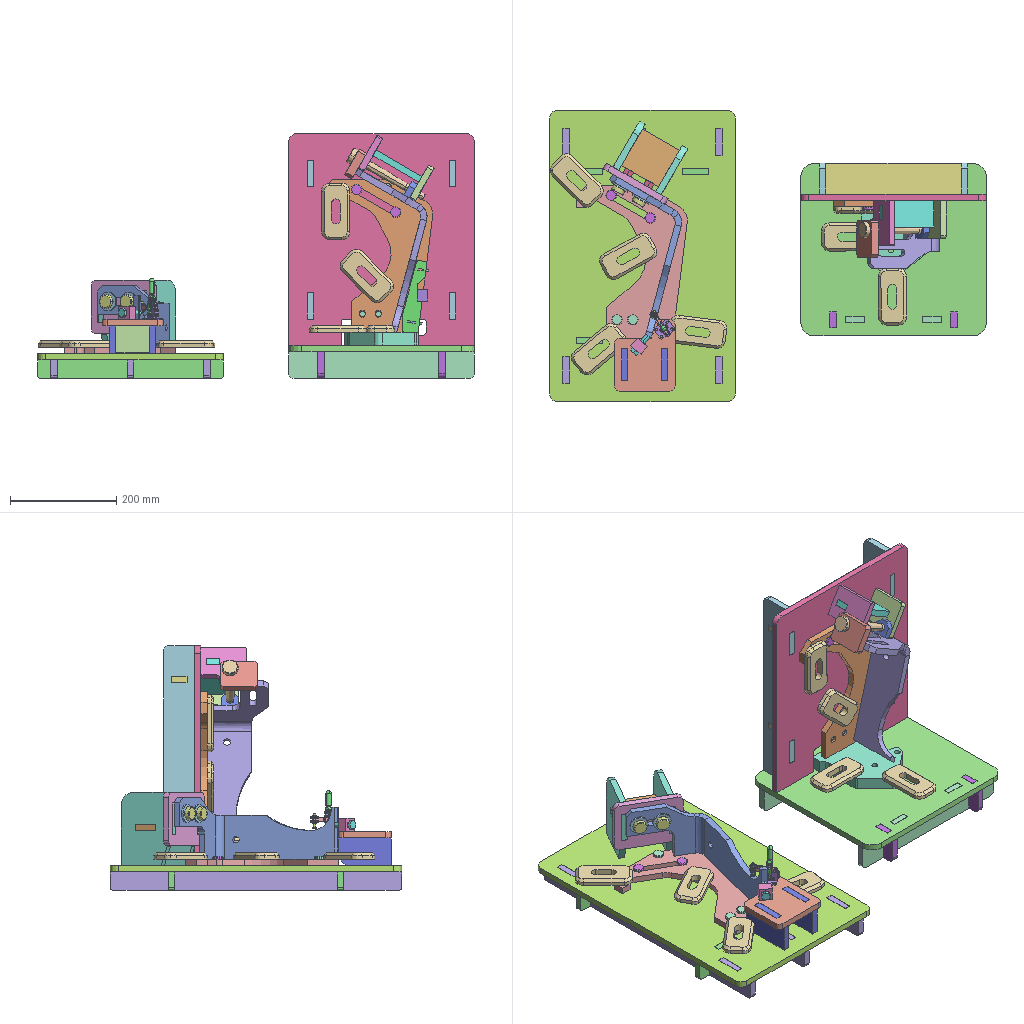Assembly | SolidWorks | 42 different items | 70 placed | box 823 x 550 x 462 mm
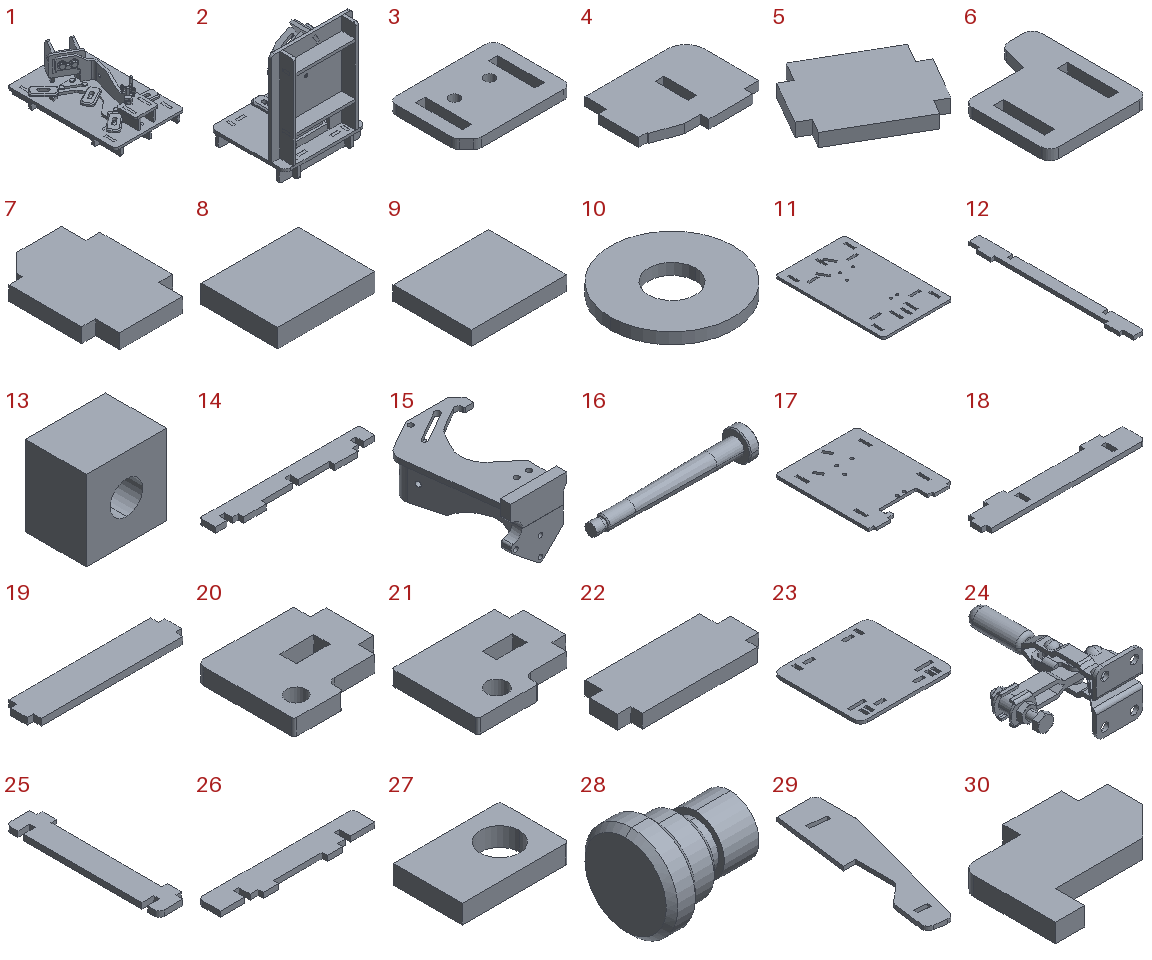Parts list (item | name | quantity | parent item | size | volume | features):
1 | (subassembly) | x1 | - | 350 x 550 x 188.62 mm | 5135552 mm3 | features InContextFeatHolder 18, ReferencePattern 9, LocalLPattern 7, CosmeticWeldCutList 1
2 | (subassembly) | x1 | - | 350 x 325 x 462 mm | 6228356 mm3 | features InContextFeatHolder 16, LocalLPattern 6, ReferencePattern 6, CosmeticWeldCutList 1
3 | - | x1 | in 1 | 134.7 x 100 x 12 mm | 138852 mm3 | features FlatPattern 1, SMBaseFlange 1, SheetMetal 1
4 | - | x2 | in 1 | 149.5 x 111.5 x 12 mm | 170572 mm3 | features FlatPattern 1, SMBaseFlange 1, SheetMetal 1
5 | - | x1 | in 1 | 112.348 x 109.632 x 12 mm | 89892 mm3 | features FlatPattern 1, SMBaseFlange 1, SheetMetal 1
6 | - | x1 | in 1 | 115 x 135 x 12 mm | 136485 mm3 | features FlatPattern 1, SMBaseFlange 1, SheetMetal 1
7 | - | x2 | in 1 | 75 x 100 x 12 mm | 77610 mm3 | features FlatPattern 1, SMBaseFlange 1, SheetMetal 1
8 | - | x1 | in 1 | 63 x 50 x 12 mm | 37800 mm3 | features FlatPattern 1, SMBaseFlange 1, SheetMetal 1
9 | - | x1 | in 1 | 80.7 x 66 x 12 mm | 63914 mm3 | features FlatPattern 1, SMBaseFlange 1, SheetMetal 1
10 | - | x2 | in 1 | 35 x 35 x 3.2 mm | 2634 mm3 | features FlatPattern 1, SMBaseFlange 1, SheetMetal 1
11 | - | x1 | in 1 | 350 x 550 x 12 mm | 2194959 mm3 | features FlatPattern 1, SMBaseFlange 1, SheetMetal 1
12 | - | x3 | in 1 | 46.5 x 550 x 12 mm | 239574 mm3 | features FlatPattern 1, SMBaseFlange 1, SheetMetal 1
13 | - | x1 | in 1 | 25 x 19 x 25 mm | 10322 mm3 | features Extrusion 1, HoleWzd 1
14 | - | x2 | in 1 | 350 x 46.5 x 12 mm | 153111 mm3 | features FlatPattern 1, SMBaseFlange 1, SheetMetal 1
15 | - | x1 | in 2 | 209.597 x 333.937 x 159.51 mm | 1061009 mm3 | features BaseBody 3
16 | - | x1 | in 2 | 160 x 30 x 30 mm | 35227 mm3 | features Chamfer 1, Revolution 1
17 | - | x1 | in 2 | 350 x 411.5 x 12 mm | 1556687 mm3 | features FlatPattern 1, SMBaseFlange 1, SheetMetal 1
18 | - | x2 | in 2 | 411.5 x 70 x 12 mm | 289842 mm3 | features FlatPattern 1, SMBaseFlange 1, SheetMetal 1
19 | - | x2 | in 2 | 279 x 58.5 x 12 mm | 187992 mm3 | features FlatPattern 1, SMBaseFlange 1, SheetMetal 1
20 | - | x1 | in 2 | 82.5 x 71.502 x 12 mm | 55316 mm3 | features FlatPattern 1, SMBaseFlange 1, SheetMetal 1
21 | - | x1 | in 2 | 96.5 x 71.502 x 12 mm | 66641 mm3 | features FlatPattern 1, SMBaseFlange 1, SheetMetal 1
22 | - | x1 | in 2 | 123 x 50 x 12 mm | 66900 mm3 | features FlatPattern 1, SMBaseFlange 1, SheetMetal 1
23 | - | x1 | in 2 | 350 x 325 x 12 mm | 1295202 mm3 | features FlatPattern 1, SMBaseFlange 1, SheetMetal 1
24 | - | x1 | in 1 | 56.45 x 77.62 x 33.3 mm | 10418 mm3 | features BaseBody 5
25 | - | x2 | in 2 | 61.5 x 325 x 12 mm | 195507 mm3 | features FlatPattern 1, SMBaseFlange 1, SheetMetal 1
26 | - | x2 | in 2 | 350 x 61.5 x 12 mm | 211887 mm3 | features FlatPattern 1, SMBaseFlange 1, SheetMetal 1
27 | - | x1 | in 2 | 34 x 22 x 6 mm | 3749 mm3 | features FlatPattern 1, SMBaseFlange 1, SheetMetal 1
28 | - | x1 | in 2 | 18 x 16 x 16 mm | 2124 mm3 | features Chamfer 1, Revolution 1
29 | - | x1 | in 2 | 46.127 x 135.184 x 3.2 mm | 10243 mm3 | features FlatPattern 1, SMBaseFlange 1, SheetMetal 1
30 | - | x1 | in 2 | 25 x 19 x 3.2 mm | 1013 mm3 | features FlatPattern 1, SMBaseFlange 1, SheetMetal 1
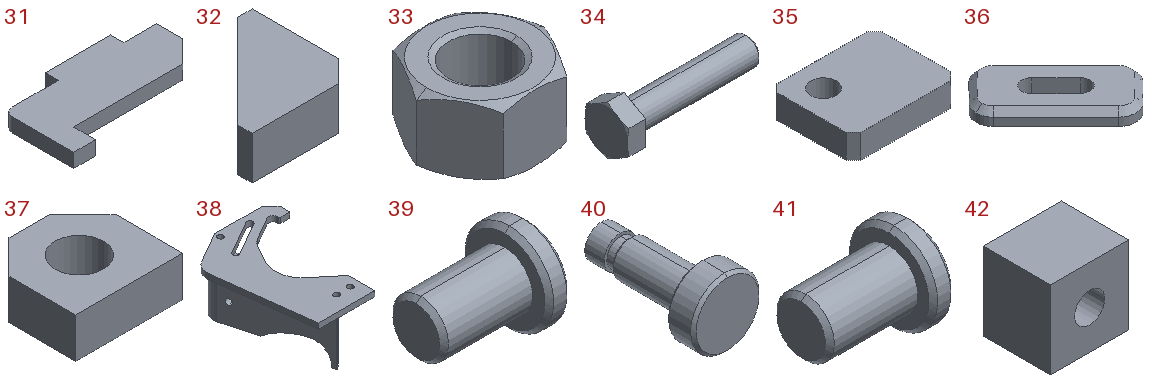31 | - | x1 | in 2 | 35 x 19 x 3.2 mm | 1413 mm3 | features FlatPattern 1, SMBaseFlange 1, SheetMetal 1
32 | - | x1 | in 2 | 15 x 15 x 6 mm | 816 mm3 | features FlatPattern 1, SMBaseFlange 1, SheetMetal 1
33 | - | x2 | in 1 | 27.713 x 24 x 14.8 mm | 5071 mm3 | features RevCut 2, Chamfer 1, Extrusion 1, LPattern 1
34 | - | x1 | in 1 | 52.08 x 15.73 x 18.163 mm | 5022 mm3 | features RevCut 2, Boss 1, Chamfer 1, Extrusion 1, Fillet 1, LPattern 1, Revolution 1
35 | - | x1 | in 2 | 70 x 56 x 16 mm | 58288 mm3 | features FlatPattern 1, SMBaseFlange 1, SheetMetal 1
36 | - | x9 | in 1, 2 | 100.711 x 100.711 x 12 mm | 53343 mm3 | features Chamfer 1, FlatPattern 1, SMBaseFlange 1, SheetMetal 1
37 | - | x1 | in 2 | 32 x 30 x 12 mm | 8338 mm3 | features FlatPattern 1, SMBaseFlange 1, SheetMetal 1
38 | - | x1 | in 1 | 209.597 x 308.937 x 128 mm | 664843 mm3 | features BaseBody 2
39 | - | x6 | in 1, 2 | 25 x 20 x 20 mm | 3946 mm3 | features Chamfer 1, Revolution 1
40 | - | x2 | in 1 | 25 x 46.2 x 25 mm | 9480 mm3 | features Chamfer 1, Revolution 1
41 | - | x4 | in 1, 2 | 25 x 20 x 20 mm | 4145 mm3 | features Chamfer 1, Revolution 1
42 | - | x1 | in 2 | 22 x 19 x 22 mm | 8118 mm3 | features BaseBody 1
Mates (type | each side: item.copy, entity, surface, feature):
In the top assembly
Coincident | 12.1 face plane Base-Flange1 | 25.1 face plane Base-Flange1
In subassembly 2
InPlace | 15.1 face plane 22U-979-5171-02.stp-1-solid1 | 23.1 plane
InPlace | 15.1 face plane 22U-979-5171-01.stp-1-solid1 | 17.1 plane
InPlace | 18.1 plane | 2.1 plane
InPlace | 19.1 plane | 2.1 plane
InPlace | 25.2 plane | 2.1 plane
InPlace | 26.1 plane | 2.1 plane
Coincident | 15.1 face plane 22U-979-5171-01.stp-1-solid1 | 36.1 face plane Base-Flange1
Coincident | 15.1 face plane 22U-979-5171-01.stp-1-solid1 | 36.2 face plane Base-Flange1
Coincident | 15.1 face plane 22U-979-5171-01.stp-1-solid1 | 36.3 face plane Base-Flange1
Coincident | 15.1 face plane 22U-979-5171-02.stp-1-solid1 | 36.4 face plane Base-Flange1
Coincident | 15.1 face plane 22U-979-5171-02.stp-1-solid1 | 36.5 face plane Base-Flange1
Concentric | 17.1 face cylinder Base-Flange1 | 39.1 face cylinder Revolve1
Coincident | 17.1 face plane Base-Flange1 | 39.1 face plane Revolve1
Concentric | 17.1 face cylinder Base-Flange1 | 39.2 face cylinder Revolve1
Coincident | 17.1 face plane Base-Flange1 | 39.2 face plane Revolve1
Coincident | 15.1 face plane 22U-979-5171-01.stp-1-solid1 | 41.1 face plane Revolve1
Concentric | 17.1 face cylinder Base-Flange1 | 41.1 face cylinder Revolve1
DistanceDim | 35.1 face plane Base-Flange1 | 15.1 face plane 22U-979-5171-03.stp-1-solid1
DistanceDim | 15.1 face plane 22U-979-5171-01.stp-1-solid1 | 35.1 face cylinder Base-Flange1
DistanceDim | 15.1 face plane 22U-979-5171-03.stp-1-solid1 | 35.1 face cylinder Base-Flange1
Parallel | 15.1 face plane 22U-979-5171-03.stp-1-solid1 | 35.1 face plane Base-Flange1
Coincident | 15.1 face plane 22U-979-5171-03.stp-1-solid1 | 37.1 face plane Base-Flange1
DistanceDim | 35.1 face plane Base-Flange1 | 37.1 face plane Base-Flange1
InPlace | 37.1 face plane Base-Flange1 | 20.1 plane
DistanceDim | 37.1 face cylinder Base-Flange1 | 15.1 face plane 22U-979-5171-01.stp-1-solid1
InPlace | 35.1 face plane Base-Flange1 | 21.1 plane
InPlace | 22.1 plane | 2.1 plane
InPlace | 16.1 plane | 2.1 plane
Coincident | 15.1 face plane 22U-979-5171-01.stp-1-solid1 | 42.1 face plane Input1
DistanceDim | 42.1 face plane Input1 | 15.1 face plane 22U-979-5171-02.stp-1-solid1
DistanceDim | 15.1 face plane 22U-979-5171-02.stp-1-solid1 | 42.1 face plane Input1
InPlace | 42.1 face plane Input1 | 27.1 plane
Coincident | 17.1 face plane Base-Flange1 | 32.1 face plane Base-Flange1
Coincident | 27.1 face plane Base-Flange1 | 32.1 face plane Base-Flange1
InPlace | 28.1 plane | 2.1 plane
InPlace | 29.1 plane | 2.1 plane
InPlace | 30.1 plane | 2.1 plane
Coincident | 15.1 face plane 22U-979-5171-01.stp-1-solid1 | 31.1 face plane Base-Flange1
Coincident | 30.1 face plane Base-Flange1 | 31.1 face plane Base-Flange1
DistanceDim | 31.1 face plane Base-Flange1 | 30.1 face plane Base-Flange1
In subassembly 1
InPlace | 38.1 face plane 22U-979-5171-01.stp-1-solid1 | 11.1 plane
InPlace | 38.1 face plane 22U-979-5171-03.stp-1-solid1 | 3.1 plane
InPlace | 4.1 plane | 1.1 plane
InPlace | 5.1 plane | 1.1 plane
InPlace | 12.2 plane | 1.1 plane
InPlace | 14.1 plane | 1.1 plane
Concentric | 3.1 face cylinder Base-Flange1 | 33.1 face cone EndChamfer
Coincident | 3.1 face plane Base-Flange1 | 33.1 face plane BaseNut
Concentric | 3.1 face cylinder Base-Flange1 | 33.2 face cone EndChamfer
Coincident | 3.1 face plane Base-Flange1 | 33.2 face plane BaseNut
InPlace | 38.1 face plane 22U-979-5171-03.stp-1-solid1 | 10.1 plane
InPlace | 40.1 plane | 1.1 plane
InPlace | 41.1 plane | 1.1 plane
InPlace | 39.1 plane | 1.1 plane
Concentric | 38.1 face cylinder 22U-979-5171-01.stp-1-solid1 | 39.3 face cylinder Revolve1
Coincident | 38.1 face plane 22U-979-5171-01.stp-1-solid1 | 39.3 face plane Revolve1
Parallel | 38.1 face plane 22U-979-5171-01.stp-1-solid1 | 39.3 plane
InPlace | 6.1 plane | 1.1 plane
InPlace | 7.1 plane | 1.1 plane
InPlace | 8.1 plane | 1.1 plane
DistanceDim | 38.1 face plane 22U-979-5171-03.stp-1-solid1 | 13.1 face plane Boss-Extrude1
Coincident | 6.1 face plane Base-Flange1 | 13.1 face plane Boss-Extrude1
Coincident | 6.1 face plane Base-Flange1 | 13.1 edge
Concentric | 13.1 face cylinder M12 Threaded Hole1 | 34.1 face cylinder BaseBody
Coincident | 13.1 face plane Boss-Extrude1 | 34.1 face plane Revolve1
InPlace | 38.1 face plane 22U-979-5171-01.stp-1-solid1 | 36.1 plane
Coincident | 38.1 face plane 22U-979-5171-01.stp-1-solid1 | 36.2 face plane Base-Flange1
DistanceDim | 38.1 face plane 22U-979-5171-01.stp-1-solid1 | 36.2 face plane Base-Flange1
DistanceDim | 36.2 face cylinder Base-Flange1 | 38.1 face plane 22U-979-5171-01.stp-1-solid1
Coincident | 38.1 face plane 22U-979-5171-01.stp-1-solid1 | 36.3 face plane Base-Flange1
DistanceDim | 36.3 face plane Base-Flange1 | 38.1 face plane 22U-979-5171-01.stp-1-solid1
DistanceDim | 36.3 face cylinder Base-Flange1 | 38.1 face plane 22U-979-5171-01.stp-1-solid1
Coincident | 38.1 face plane 22U-979-5171-01.stp-1-solid1 | 36.4 face plane Base-Flange1
DistanceDim | 38.1 face plane 22U-979-5171-01.stp-1-solid1 | 36.4 face plane Base-Flange1
DistanceDim | 36.4 face cylinder Base-Flange1 | 38.1 face plane 22U-979-5171-01.stp-1-solid1
Coincident | 6.1 face plane Base-Flange1 | 24.1 face plane TC1-1 vertical flange-base toggle clamp[TCS1-1].step-1/_TCS1-1(seat).step-1-solid1
PlanarAngleDim | 24.1 face plane TC1-1 vertical flange-base toggle clamp[TCS1-1].step-1/_TCS1-1(seat).step-1-solid1 | 6.1 face plane Base-Flange1
DistanceDim | 24.1 face cylinder TC1-1 vertical flange-base toggle clamp[TCS1-1].step-1/_TCS1-1(seat).step-1-solid1 | 6.1 face plane Base-Flange1
DistanceDim | 6.1 face plane Base-Flange1 | 24.1 face cylinder TC1-1 vertical flange-base toggle clamp[TCS1-1].step-1/_TCS1-1(seat).step-1-solid1
InPlace | 5.1 face plane Base-Flange1 | 9.1 plane